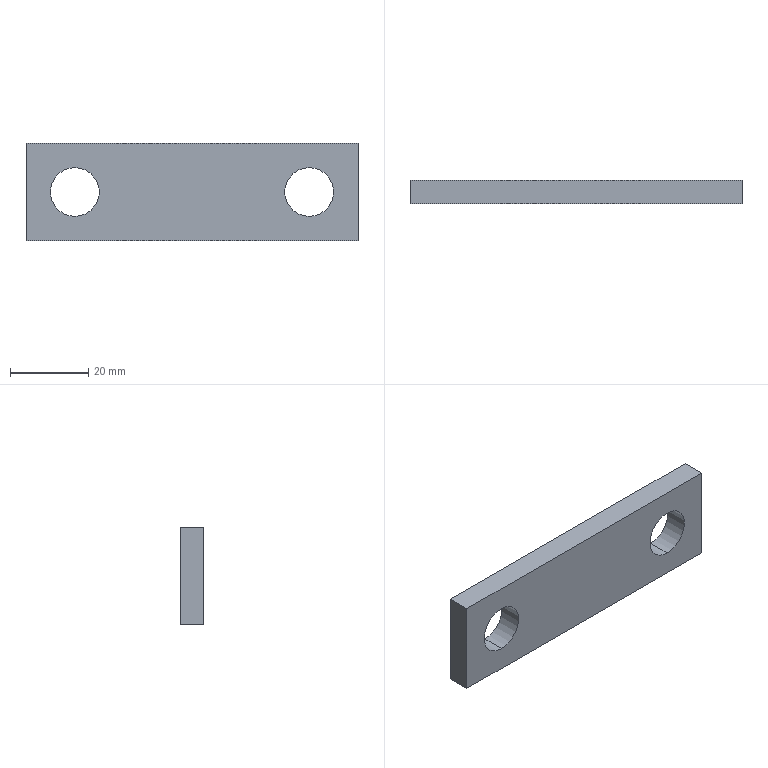Part | SolidWorks | features FlatPattern 1, SMBaseFlange 1, SheetMetal 1 | 1 solid | 10 faces | box 85 x 6 x 25 mm | volume 11277 mm3 | plane 6 | cylinder 4 | commonest cylinder face diameters 12.5 x4
STEP:
#1=CARTESIAN_POINT('',(72.5,-6.,6.25));
#2=VERTEX_POINT('',#1);
#3=CARTESIAN_POINT('',(72.5,-6.,18.75));
#4=VERTEX_POINT('',#3);
#5=CARTESIAN_POINT('',(72.5,-6.,12.5));
#6=DIRECTION('',(0.,1.,0.));
#7=DIRECTION('',(0.,0.,1.));
#8=AXIS2_PLACEMENT_3D('',#5,#6,#7);
#9=CIRCLE('',#8,6.25);
#10=EDGE_CURVE('',#2,#4,#9,.T.);
#11=ORIENTED_EDGE('',*,*,#10,.F.);
#12=CARTESIAN_POINT('',(72.5,0.,6.25));
#13=VERTEX_POINT('',#12);
#14=CARTESIAN_POINT('',(72.5,-6.,6.25));
#15=DIRECTION('',(0.,1.,0.));
#16=VECTOR('',#15,1000.);
#17=LINE('',#14,#16);
#18=EDGE_CURVE('',#2,#13,#17,.T.);
#19=ORIENTED_EDGE('',*,*,#18,.T.);
#20=CARTESIAN_POINT('',(72.5,0.,18.75));
#21=VERTEX_POINT('',#20);
#22=CARTESIAN_POINT('',(72.5,0.,12.5));
#23=DIRECTION('',(0.,1.,0.));
#24=DIRECTION('',(0.,0.,1.));
#25=AXIS2_PLACEMENT_3D('',#22,#23,#24);
#26=CIRCLE('',#25,6.25);
#27=EDGE_CURVE('',#13,#21,#26,.T.);
#28=ORIENTED_EDGE('',*,*,#27,.T.);
#29=CARTESIAN_POINT('',(72.5,-6.,18.75));
#30=DIRECTION('',(0.,1.,0.));
#31=VECTOR('',#30,1000.);
#32=LINE('',#29,#31);
#33=EDGE_CURVE('',#4,#21,#32,.T.);
#34=ORIENTED_EDGE('',*,*,#33,.F.);
#35=EDGE_LOOP('',(#11,#19,#28,#34));
#36=FACE_OUTER_BOUND('',#35,.T.);
#37=CARTESIAN_POINT('',(72.5,-6.,12.5));
#38=DIRECTION('',(0.,1.,0.));
#39=DIRECTION('',(0.,0.,1.));
#40=AXIS2_PLACEMENT_3D('',#37,#38,#39);
#41=CYLINDRICAL_SURFACE('',#40,6.25);
#42=ADVANCED_FACE('',(#36),#41,.F.);
#43=CARTESIAN_POINT('',(12.5,-6.,6.25));
#44=VERTEX_POINT('',#43);
#45=CARTESIAN_POINT('',(12.5,-6.,18.75));
#46=VERTEX_POINT('',#45);
#47=CARTESIAN_POINT('',(12.5,-6.,12.5));
#48=DIRECTION('',(0.,1.,0.));
#49=DIRECTION('',(0.,0.,1.));
#50=AXIS2_PLACEMENT_3D('',#47,#48,#49);
#51=CIRCLE('',#50,6.25);
#52=EDGE_CURVE('',#44,#46,#51,.T.);
#53=ORIENTED_EDGE('',*,*,#52,.F.);
#54=CARTESIAN_POINT('',(12.5,0.,6.25));
#55=VERTEX_POINT('',#54);
#56=CARTESIAN_POINT('',(12.5,-6.,6.25));
#57=DIRECTION('',(0.,1.,0.));
#58=VECTOR('',#57,1000.);
#59=LINE('',#56,#58);
#60=EDGE_CURVE('',#44,#55,#59,.T.);
#61=ORIENTED_EDGE('',*,*,#60,.T.);
#62=CARTESIAN_POINT('',(12.5,0.,18.75));
#63=VERTEX_POINT('',#62);
#64=CARTESIAN_POINT('',(12.5,0.,12.5));
#65=DIRECTION('',(0.,1.,0.));
#66=DIRECTION('',(0.,0.,1.));
#67=AXIS2_PLACEMENT_3D('',#64,#65,#66);
#68=CIRCLE('',#67,6.25);
#69=EDGE_CURVE('',#55,#63,#68,.T.);
#70=ORIENTED_EDGE('',*,*,#69,.T.);
#71=CARTESIAN_POINT('',(12.5,-6.,18.75));
#72=DIRECTION('',(0.,1.,0.));
#73=VECTOR('',#72,1000.);
#74=LINE('',#71,#73);
#75=EDGE_CURVE('',#46,#63,#74,.T.);
#76=ORIENTED_EDGE('',*,*,#75,.F.);
#77=EDGE_LOOP('',(#53,#61,#70,#76));
#78=FACE_OUTER_BOUND('',#77,.T.);
#79=CARTESIAN_POINT('',(12.5,-6.,12.5));
#80=DIRECTION('',(0.,1.,0.));
#81=DIRECTION('',(0.,0.,1.));
#82=AXIS2_PLACEMENT_3D('',#79,#80,#81);
#83=CYLINDRICAL_SURFACE('',#82,6.25);
#84=ADVANCED_FACE('',(#78),#83,.F.);
#85=CARTESIAN_POINT('',(0.,0.,0.));
#86=VERTEX_POINT('',#85);
#87=CARTESIAN_POINT('',(0.,0.,25.));
#88=VERTEX_POINT('',#87);
#89=CARTESIAN_POINT('',(0.,0.,0.));
#90=DIRECTION('',(0.,0.,1.));
#91=VECTOR('',#90,1000.);
#92=LINE('',#89,#91);
#93=EDGE_CURVE('',#86,#88,#92,.T.);
#94=ORIENTED_EDGE('',*,*,#93,.F.);
#95=CARTESIAN_POINT('',(0.,-6.,0.));
#96=VERTEX_POINT('',#95);
#97=CARTESIAN_POINT('',(0.,-6.,0.));
#98=DIRECTION('',(0.,1.,0.));
#99=VECTOR('',#98,1000.);
#100=LINE('',#97,#99);
#101=EDGE_CURVE('',#96,#86,#100,.T.);
#102=ORIENTED_EDGE('',*,*,#101,.F.);
#103=CARTESIAN_POINT('',(0.,-6.,25.));
#104=VERTEX_POINT('',#103);
#105=CARTESIAN_POINT('',(0.,-6.,0.));
#106=DIRECTION('',(0.,0.,1.));
#107=VECTOR('',#106,1000.);
#108=LINE('',#105,#107);
#109=EDGE_CURVE('',#96,#104,#108,.T.);
#110=ORIENTED_EDGE('',*,*,#109,.T.);
#111=CARTESIAN_POINT('',(0.,-6.,25.));
#112=DIRECTION('',(0.,1.,0.));
#113=VECTOR('',#112,1000.);
#114=LINE('',#111,#113);
#115=EDGE_CURVE('',#104,#88,#114,.T.);
#116=ORIENTED_EDGE('',*,*,#115,.T.);
#117=EDGE_LOOP('',(#94,#102,#110,#116));
#118=FACE_OUTER_BOUND('',#117,.T.);
#119=CARTESIAN_POINT('',(0.,-6.,0.));
#120=DIRECTION('',(-1.,0.,0.));
#121=DIRECTION('',(0.,0.,1.));
#122=AXIS2_PLACEMENT_3D('',#119,#120,#121);
#123=PLANE('',#122);
#124=ADVANCED_FACE('',(#118),#123,.T.);
#125=CARTESIAN_POINT('',(85.,0.,0.));
#126=VERTEX_POINT('',#125);
#127=CARTESIAN_POINT('',(0.,0.,0.));
#128=DIRECTION('',(-1.,0.,0.));
#129=VECTOR('',#128,1000.);
#130=LINE('',#127,#129);
#131=EDGE_CURVE('',#126,#86,#130,.T.);
#132=ORIENTED_EDGE('',*,*,#131,.F.);
#133=CARTESIAN_POINT('',(85.,-6.,0.));
#134=VERTEX_POINT('',#133);
#135=CARTESIAN_POINT('',(85.,-6.,0.));
#136=DIRECTION('',(0.,1.,0.));
#137=VECTOR('',#136,1000.);
#138=LINE('',#135,#137);
#139=EDGE_CURVE('',#134,#126,#138,.T.);
#140=ORIENTED_EDGE('',*,*,#139,.F.);
#141=CARTESIAN_POINT('',(0.,-6.,0.));
#142=DIRECTION('',(-1.,0.,0.));
#143=VECTOR('',#142,1000.);
#144=LINE('',#141,#143);
#145=EDGE_CURVE('',#134,#96,#144,.T.);
#146=ORIENTED_EDGE('',*,*,#145,.T.);
#147=ORIENTED_EDGE('',*,*,#101,.T.);
#148=EDGE_LOOP('',(#132,#140,#146,#147));
#149=FACE_OUTER_BOUND('',#148,.T.);
#150=CARTESIAN_POINT('',(0.,-6.,0.));
#151=DIRECTION('',(0.,0.,-1.));
#152=DIRECTION('',(-1.,0.,0.));
#153=AXIS2_PLACEMENT_3D('',#150,#151,#152);
#154=PLANE('',#153);
#155=ADVANCED_FACE('',(#149),#154,.T.);
#156=CARTESIAN_POINT('',(85.,0.,25.));
#157=VERTEX_POINT('',#156);
#158=CARTESIAN_POINT('',(85.,0.,0.));
#159=DIRECTION('',(0.,0.,-1.));
#160=VECTOR('',#159,1000.);
#161=LINE('',#158,#160);
#162=EDGE_CURVE('',#157,#126,#161,.T.);
#163=ORIENTED_EDGE('',*,*,#162,.F.);
#164=CARTESIAN_POINT('',(85.,-6.,25.));
#165=VERTEX_POINT('',#164);
#166=CARTESIAN_POINT('',(85.,-6.,25.));
#167=DIRECTION('',(0.,1.,0.));
#168=VECTOR('',#167,1000.);
#169=LINE('',#166,#168);
#170=EDGE_CURVE('',#165,#157,#169,.T.);
#171=ORIENTED_EDGE('',*,*,#170,.F.);
#172=CARTESIAN_POINT('',(85.,-6.,0.));
#173=DIRECTION('',(0.,0.,-1.));
#174=VECTOR('',#173,1000.);
#175=LINE('',#172,#174);
#176=EDGE_CURVE('',#165,#134,#175,.T.);
#177=ORIENTED_EDGE('',*,*,#176,.T.);
#178=ORIENTED_EDGE('',*,*,#139,.T.);
#179=EDGE_LOOP('',(#163,#171,#177,#178));
#180=FACE_OUTER_BOUND('',#179,.T.);
#181=CARTESIAN_POINT('',(85.,-6.,0.));
#182=DIRECTION('',(1.,0.,0.));
#183=DIRECTION('',(0.,0.,-1.));
#184=AXIS2_PLACEMENT_3D('',#181,#182,#183);
#185=PLANE('',#184);
#186=ADVANCED_FACE('',(#180),#185,.T.);
#187=CARTESIAN_POINT('',(0.,0.,25.));
#188=DIRECTION('',(1.,0.,0.));
#189=VECTOR('',#188,1000.);
#190=LINE('',#187,#189);
#191=EDGE_CURVE('',#88,#157,#190,.T.);
#192=ORIENTED_EDGE('',*,*,#191,.F.);
#193=ORIENTED_EDGE('',*,*,#115,.F.);
#194=CARTESIAN_POINT('',(0.,-6.,25.));
#195=DIRECTION('',(1.,0.,0.));
#196=VECTOR('',#195,1000.);
#197=LINE('',#194,#196);
#198=EDGE_CURVE('',#104,#165,#197,.T.);
#199=ORIENTED_EDGE('',*,*,#198,.T.);
#200=ORIENTED_EDGE('',*,*,#170,.T.);
#201=EDGE_LOOP('',(#192,#193,#199,#200));
#202=FACE_OUTER_BOUND('',#201,.T.);
#203=CARTESIAN_POINT('',(0.,-6.,25.));
#204=DIRECTION('',(0.,0.,1.));
#205=DIRECTION('',(1.,0.,0.));
#206=AXIS2_PLACEMENT_3D('',#203,#204,#205);
#207=PLANE('',#206);
#208=ADVANCED_FACE('',(#202),#207,.T.);
#209=CARTESIAN_POINT('',(72.5,-6.,12.5));
#210=DIRECTION('',(0.,1.,0.));
#211=DIRECTION('',(0.,0.,1.));
#212=AXIS2_PLACEMENT_3D('',#209,#210,#211);
#213=CIRCLE('',#212,6.25);
#214=EDGE_CURVE('',#4,#2,#213,.T.);
#215=ORIENTED_EDGE('',*,*,#214,.T.);
#216=ORIENTED_EDGE('',*,*,#10,.T.);
#217=EDGE_LOOP('',(#215,#216));
#218=FACE_BOUND('',#217,.T.);
#219=CARTESIAN_POINT('',(12.5,-6.,12.5));
#220=DIRECTION('',(0.,1.,0.));
#221=DIRECTION('',(0.,0.,1.));
#222=AXIS2_PLACEMENT_3D('',#219,#220,#221);
#223=CIRCLE('',#222,6.25);
#224=EDGE_CURVE('',#46,#44,#223,.T.);
#225=ORIENTED_EDGE('',*,*,#224,.T.);
#226=ORIENTED_EDGE('',*,*,#52,.T.);
#227=EDGE_LOOP('',(#225,#226));
#228=FACE_BOUND('',#227,.T.);
#229=ORIENTED_EDGE('',*,*,#109,.F.);
#230=ORIENTED_EDGE('',*,*,#145,.F.);
#231=ORIENTED_EDGE('',*,*,#176,.F.);
#232=ORIENTED_EDGE('',*,*,#198,.F.);
#233=EDGE_LOOP('',(#229,#230,#231,#232));
#234=FACE_OUTER_BOUND('',#233,.T.);
#235=CARTESIAN_POINT('',(0.,-6.,0.));
#236=DIRECTION('',(0.,1.,0.));
#237=DIRECTION('',(0.,0.,1.));
#238=AXIS2_PLACEMENT_3D('',#235,#236,#237);
#239=PLANE('',#238);
#240=ADVANCED_FACE('',(#218,#228,#234),#239,.F.);
#241=CARTESIAN_POINT('',(72.5,0.,12.5));
#242=DIRECTION('',(0.,1.,0.));
#243=DIRECTION('',(0.,0.,1.));
#244=AXIS2_PLACEMENT_3D('',#241,#242,#243);
#245=CIRCLE('',#244,6.25);
#246=EDGE_CURVE('',#21,#13,#245,.T.);
#247=ORIENTED_EDGE('',*,*,#246,.F.);
#248=ORIENTED_EDGE('',*,*,#27,.F.);
#249=EDGE_LOOP('',(#247,#248));
#250=FACE_BOUND('',#249,.T.);
#251=CARTESIAN_POINT('',(12.5,0.,12.5));
#252=DIRECTION('',(0.,1.,0.));
#253=DIRECTION('',(0.,0.,1.));
#254=AXIS2_PLACEMENT_3D('',#251,#252,#253);
#255=CIRCLE('',#254,6.25);
#256=EDGE_CURVE('',#63,#55,#255,.T.);
#257=ORIENTED_EDGE('',*,*,#256,.F.);
#258=ORIENTED_EDGE('',*,*,#69,.F.);
#259=EDGE_LOOP('',(#257,#258));
#260=FACE_BOUND('',#259,.T.);
#261=ORIENTED_EDGE('',*,*,#93,.T.);
#262=ORIENTED_EDGE('',*,*,#191,.T.);
#263=ORIENTED_EDGE('',*,*,#162,.T.);
#264=ORIENTED_EDGE('',*,*,#131,.T.);
#265=EDGE_LOOP('',(#261,#262,#263,#264));
#266=FACE_OUTER_BOUND('',#265,.T.);
#267=CARTESIAN_POINT('',(0.,0.,0.));
#268=DIRECTION('',(0.,1.,0.));
#269=DIRECTION('',(0.,0.,1.));
#270=AXIS2_PLACEMENT_3D('',#267,#268,#269);
#271=PLANE('',#270);
#272=ADVANCED_FACE('',(#250,#260,#266),#271,.T.);
#273=ORIENTED_EDGE('',*,*,#60,.F.);
#274=ORIENTED_EDGE('',*,*,#224,.F.);
#275=ORIENTED_EDGE('',*,*,#75,.T.);
#276=ORIENTED_EDGE('',*,*,#256,.T.);
#277=EDGE_LOOP('',(#273,#274,#275,#276));
#278=FACE_OUTER_BOUND('',#277,.T.);
#279=CARTESIAN_POINT('',(12.5,-6.,12.5));
#280=DIRECTION('',(0.,1.,0.));
#281=DIRECTION('',(0.,0.,1.));
#282=AXIS2_PLACEMENT_3D('',#279,#280,#281);
#283=CYLINDRICAL_SURFACE('',#282,6.25);
#284=ADVANCED_FACE('',(#278),#283,.F.);
#285=ORIENTED_EDGE('',*,*,#18,.F.);
#286=ORIENTED_EDGE('',*,*,#214,.F.);
#287=ORIENTED_EDGE('',*,*,#33,.T.);
#288=ORIENTED_EDGE('',*,*,#246,.T.);
#289=EDGE_LOOP('',(#285,#286,#287,#288));
#290=FACE_OUTER_BOUND('',#289,.T.);
#291=CARTESIAN_POINT('',(72.5,-6.,12.5));
#292=DIRECTION('',(0.,1.,0.));
#293=DIRECTION('',(0.,0.,1.));
#294=AXIS2_PLACEMENT_3D('',#291,#292,#293);
#295=CYLINDRICAL_SURFACE('',#294,6.25);
#296=ADVANCED_FACE('',(#290),#295,.F.);
#297=CLOSED_SHELL('',(#42,#84,#124,#155,#186,#208,#240,#272,#284,#296));
#298=MANIFOLD_SOLID_BREP('',#297);
#299=CARTESIAN_POINT('',(0.,0.,0.));
#300=DIRECTION('',(0.,0.,1.));
#301=DIRECTION('',(1.,0.,0.));
#302=AXIS2_PLACEMENT_3D('',#299,#300,#301);
#303=(LENGTH_UNIT()NAMED_UNIT(*)SI_UNIT(.MILLI.,.METRE.));
#304=UNCERTAINTY_MEASURE_WITH_UNIT(LENGTH_MEASURE(0.00001),#303,'','');
#305=(NAMED_UNIT(*)PLANE_ANGLE_UNIT()SI_UNIT($,.RADIAN.));
#306=(NAMED_UNIT(*)SI_UNIT($,.STERADIAN.)SOLID_ANGLE_UNIT());
#307=(GEOMETRIC_REPRESENTATION_CONTEXT(3)GLOBAL_UNCERTAINTY_ASSIGNED_CONTEXT((#304))GLOBAL_UNIT_ASSIGNED_CONTEXT((#303,#305,#306))REPRESENTATION_CONTEXT('',''));
#308=ADVANCED_BREP_SHAPE_REPRESENTATION('',(#298,#302),#307);